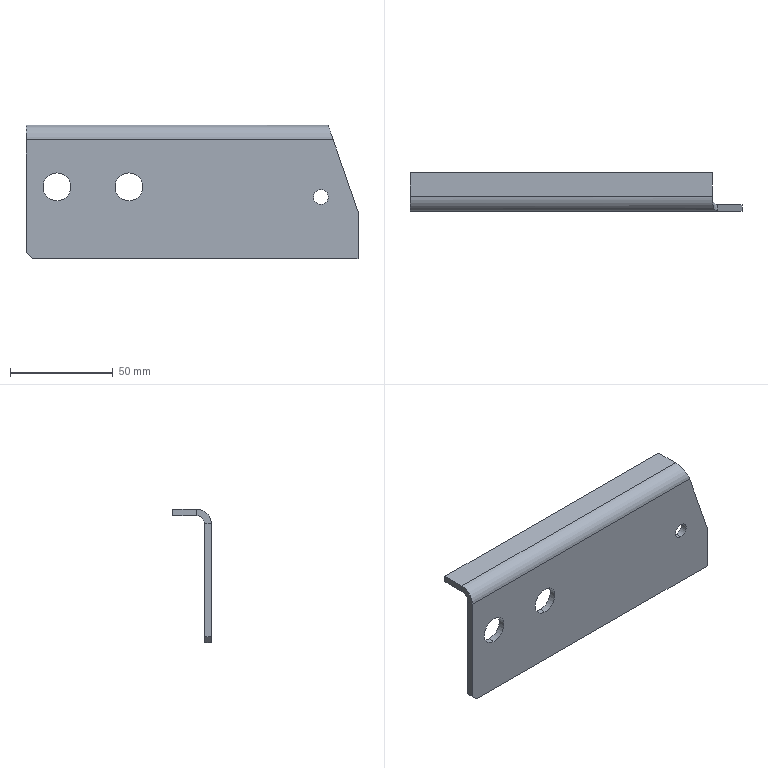Part | SolidWorks | features ICE 3, BreakCorner 1, EdgeFlange 1, FlatPattern 1, SMBaseFlange 1, SheetMetal 1 | 1 solid | 22 faces | box 161.2 x 18.8 x 65 mm | volume 37684 mm3 | plane 13 | cylinder 8 | spline 1 | commonest cylinder face diameters 13.5 x4 7.2 x2 8 x1 14.4 x1
STEP:
#1=CARTESIAN_POINT('',(62.6,-3.2,-6.1));
#2=VERTEX_POINT('',#1);
#3=CARTESIAN_POINT('',(62.6,-3.2,1.1));
#4=VERTEX_POINT('',#3);
#5=CARTESIAN_POINT('',(62.6,-3.2,-2.5));
#6=DIRECTION('',(0.,1.,0.));
#7=DIRECTION('',(0.,0.,1.));
#8=AXIS2_PLACEMENT_3D('',#5,#6,#7);
#9=CIRCLE('',#8,3.6);
#10=EDGE_CURVE('',#2,#4,#9,.T.);
#11=ORIENTED_EDGE('',*,*,#10,.F.);
#12=CARTESIAN_POINT('',(62.6,0.,-6.1));
#13=VERTEX_POINT('',#12);
#14=CARTESIAN_POINT('',(62.6,-10.,-6.1));
#15=DIRECTION('',(0.,1.,0.));
#16=VECTOR('',#15,1000.);
#17=LINE('',#14,#16);
#18=EDGE_CURVE('',#2,#13,#17,.T.);
#19=ORIENTED_EDGE('',*,*,#18,.T.);
#20=CARTESIAN_POINT('',(62.6,0.,1.1));
#21=VERTEX_POINT('',#20);
#22=CARTESIAN_POINT('',(62.6,0.,-2.5));
#23=DIRECTION('',(0.,1.,0.));
#24=DIRECTION('',(0.,0.,1.));
#25=AXIS2_PLACEMENT_3D('',#22,#23,#24);
#26=CIRCLE('',#25,3.6);
#27=EDGE_CURVE('',#13,#21,#26,.T.);
#28=ORIENTED_EDGE('',*,*,#27,.T.);
#29=CARTESIAN_POINT('',(62.6,-10.,1.1));
#30=DIRECTION('',(0.,1.,0.));
#31=VECTOR('',#30,1000.);
#32=LINE('',#29,#31);
#33=EDGE_CURVE('',#4,#21,#32,.T.);
#34=ORIENTED_EDGE('',*,*,#33,.F.);
#35=EDGE_LOOP('',(#11,#19,#28,#34));
#36=FACE_OUTER_BOUND('',#35,.T.);
#37=CARTESIAN_POINT('',(62.6,-10.,-2.5));
#38=DIRECTION('',(0.,1.,0.));
#39=DIRECTION('',(0.,0.,1.));
#40=AXIS2_PLACEMENT_3D('',#37,#38,#39);
#41=CYLINDRICAL_SURFACE('',#40,3.6);
#42=ADVANCED_FACE('',(#36),#41,.F.);
#43=CARTESIAN_POINT('',(-30.6,-3.2,-4.25));
#44=VERTEX_POINT('',#43);
#45=CARTESIAN_POINT('',(-30.6,-3.2,9.25));
#46=VERTEX_POINT('',#45);
#47=CARTESIAN_POINT('',(-30.6,-3.2,2.5));
#48=DIRECTION('',(0.,1.,0.));
#49=DIRECTION('',(0.,0.,1.));
#50=AXIS2_PLACEMENT_3D('',#47,#48,#49);
#51=CIRCLE('',#50,6.75);
#52=EDGE_CURVE('',#44,#46,#51,.T.);
#53=ORIENTED_EDGE('',*,*,#52,.F.);
#54=CARTESIAN_POINT('',(-30.6,0.,-4.25));
#55=VERTEX_POINT('',#54);
#56=CARTESIAN_POINT('',(-30.6,-10.,-4.25));
#57=DIRECTION('',(0.,1.,0.));
#58=VECTOR('',#57,1000.);
#59=LINE('',#56,#58);
#60=EDGE_CURVE('',#44,#55,#59,.T.);
#61=ORIENTED_EDGE('',*,*,#60,.T.);
#62=CARTESIAN_POINT('',(-30.6,0.,9.25));
#63=VERTEX_POINT('',#62);
#64=CARTESIAN_POINT('',(-30.6,0.,2.5));
#65=DIRECTION('',(0.,1.,0.));
#66=DIRECTION('',(0.,0.,1.));
#67=AXIS2_PLACEMENT_3D('',#64,#65,#66);
#68=CIRCLE('',#67,6.75);
#69=EDGE_CURVE('',#55,#63,#68,.T.);
#70=ORIENTED_EDGE('',*,*,#69,.T.);
#71=CARTESIAN_POINT('',(-30.6,-10.,9.25));
#72=DIRECTION('',(0.,1.,0.));
#73=VECTOR('',#72,1000.);
#74=LINE('',#71,#73);
#75=EDGE_CURVE('',#46,#63,#74,.T.);
#76=ORIENTED_EDGE('',*,*,#75,.F.);
#77=EDGE_LOOP('',(#53,#61,#70,#76));
#78=FACE_OUTER_BOUND('',#77,.T.);
#79=CARTESIAN_POINT('',(-30.6,-10.,2.5));
#80=DIRECTION('',(0.,1.,0.));
#81=DIRECTION('',(0.,0.,1.));
#82=AXIS2_PLACEMENT_3D('',#79,#80,#81);
#83=CYLINDRICAL_SURFACE('',#82,6.75);
#84=ADVANCED_FACE('',(#78),#83,.F.);
#85=CARTESIAN_POINT('',(-65.6,-3.2,-4.25));
#86=VERTEX_POINT('',#85);
#87=CARTESIAN_POINT('',(-65.6,-3.2,9.25));
#88=VERTEX_POINT('',#87);
#89=CARTESIAN_POINT('',(-65.6,-3.2,2.5));
#90=DIRECTION('',(0.,1.,0.));
#91=DIRECTION('',(0.,0.,1.));
#92=AXIS2_PLACEMENT_3D('',#89,#90,#91);
#93=CIRCLE('',#92,6.75);
#94=EDGE_CURVE('',#86,#88,#93,.T.);
#95=ORIENTED_EDGE('',*,*,#94,.F.);
#96=CARTESIAN_POINT('',(-65.6,0.,-4.25));
#97=VERTEX_POINT('',#96);
#98=CARTESIAN_POINT('',(-65.6,-10.,-4.25));
#99=DIRECTION('',(0.,1.,0.));
#100=VECTOR('',#99,1000.);
#101=LINE('',#98,#100);
#102=EDGE_CURVE('',#86,#97,#101,.T.);
#103=ORIENTED_EDGE('',*,*,#102,.T.);
#104=CARTESIAN_POINT('',(-65.6,0.,9.25));
#105=VERTEX_POINT('',#104);
#106=CARTESIAN_POINT('',(-65.6,0.,2.5));
#107=DIRECTION('',(0.,1.,0.));
#108=DIRECTION('',(0.,0.,1.));
#109=AXIS2_PLACEMENT_3D('',#106,#107,#108);
#110=CIRCLE('',#109,6.75);
#111=EDGE_CURVE('',#97,#105,#110,.T.);
#112=ORIENTED_EDGE('',*,*,#111,.T.);
#113=CARTESIAN_POINT('',(-65.6,-10.,9.25));
#114=DIRECTION('',(0.,1.,0.));
#115=VECTOR('',#114,1000.);
#116=LINE('',#113,#115);
#117=EDGE_CURVE('',#88,#105,#116,.T.);
#118=ORIENTED_EDGE('',*,*,#117,.F.);
#119=EDGE_LOOP('',(#95,#103,#112,#118));
#120=FACE_OUTER_BOUND('',#119,.T.);
#121=CARTESIAN_POINT('',(-65.6,-10.,2.5));
#122=DIRECTION('',(0.,1.,0.));
#123=DIRECTION('',(0.,0.,1.));
#124=AXIS2_PLACEMENT_3D('',#121,#122,#123);
#125=CYLINDRICAL_SURFACE('',#124,6.75);
#126=ADVANCED_FACE('',(#120),#125,.F.);
#127=CARTESIAN_POINT('',(80.6,0.,-9.6));
#128=VERTEX_POINT('',#127);
#129=CARTESIAN_POINT('',(80.6,0.,-32.5));
#130=VERTEX_POINT('',#129);
#131=CARTESIAN_POINT('',(80.6,0.,-32.5));
#132=DIRECTION('',(0.,0.,-1.));
#133=VECTOR('',#132,1000.);
#134=LINE('',#131,#133);
#135=EDGE_CURVE('',#128,#130,#134,.T.);
#136=ORIENTED_EDGE('',*,*,#135,.F.);
#137=CARTESIAN_POINT('',(80.6,-3.2,-9.6));
#138=VERTEX_POINT('',#137);
#139=CARTESIAN_POINT('',(80.6,0.,-9.6));
#140=DIRECTION('',(0.,-1.,0.));
#141=VECTOR('',#140,1000.);
#142=LINE('',#139,#141);
#143=EDGE_CURVE('',#128,#138,#142,.T.);
#144=ORIENTED_EDGE('',*,*,#143,.T.);
#145=CARTESIAN_POINT('',(80.6,-3.2,-32.5));
#146=VERTEX_POINT('',#145);
#147=CARTESIAN_POINT('',(80.6,-3.2,-32.5));
#148=DIRECTION('',(0.,0.,-1.));
#149=VECTOR('',#148,1000.);
#150=LINE('',#147,#149);
#151=EDGE_CURVE('',#138,#146,#150,.T.);
#152=ORIENTED_EDGE('',*,*,#151,.T.);
#153=CARTESIAN_POINT('',(80.6,-3.2,-32.5));
#154=DIRECTION('',(0.,1.,0.));
#155=VECTOR('',#154,1000.);
#156=LINE('',#153,#155);
#157=EDGE_CURVE('',#146,#130,#156,.T.);
#158=ORIENTED_EDGE('',*,*,#157,.T.);
#159=EDGE_LOOP('',(#136,#144,#152,#158));
#160=FACE_OUTER_BOUND('',#159,.T.);
#161=CARTESIAN_POINT('',(80.6,-3.2,-32.5));
#162=DIRECTION('',(1.,0.,0.));
#163=DIRECTION('',(0.,0.,-1.));
#164=AXIS2_PLACEMENT_3D('',#161,#162,#163);
#165=PLANE('',#164);
#166=ADVANCED_FACE('',(#160),#165,.T.);
#167=CARTESIAN_POINT('',(62.6,-3.2,-2.5));
#168=DIRECTION('',(0.,1.,0.));
#169=DIRECTION('',(0.,0.,1.));
#170=AXIS2_PLACEMENT_3D('',#167,#168,#169);
#171=CIRCLE('',#170,3.6);
#172=EDGE_CURVE('',#4,#2,#171,.T.);
#173=ORIENTED_EDGE('',*,*,#172,.T.);
#174=ORIENTED_EDGE('',*,*,#10,.T.);
#175=EDGE_LOOP('',(#173,#174));
#176=FACE_BOUND('',#175,.T.);
#177=CARTESIAN_POINT('',(-65.6,-3.2,2.5));
#178=DIRECTION('',(0.,1.,0.));
#179=DIRECTION('',(0.,0.,1.));
#180=AXIS2_PLACEMENT_3D('',#177,#178,#179);
#181=CIRCLE('',#180,6.75);
#182=EDGE_CURVE('',#88,#86,#181,.T.);
#183=ORIENTED_EDGE('',*,*,#182,.T.);
#184=ORIENTED_EDGE('',*,*,#94,.T.);
#185=EDGE_LOOP('',(#183,#184));
#186=FACE_BOUND('',#185,.T.);
#187=CARTESIAN_POINT('',(-30.6,-3.2,2.5));
#188=DIRECTION('',(0.,1.,0.));
#189=DIRECTION('',(0.,0.,1.));
#190=AXIS2_PLACEMENT_3D('',#187,#188,#189);
#191=CIRCLE('',#190,6.75);
#192=EDGE_CURVE('',#46,#44,#191,.T.);
#193=ORIENTED_EDGE('',*,*,#192,.T.);
#194=ORIENTED_EDGE('',*,*,#52,.T.);
#195=EDGE_LOOP('',(#193,#194));
#196=FACE_BOUND('',#195,.T.);
#197=CARTESIAN_POINT('',(-80.6,-3.2,-29.5));
#198=VERTEX_POINT('',#197);
#199=CARTESIAN_POINT('',(-80.6,-3.2,25.3));
#200=VERTEX_POINT('',#199);
#201=CARTESIAN_POINT('',(-80.6,-3.2,-32.5));
#202=DIRECTION('',(0.,0.,1.));
#203=VECTOR('',#202,1000.);
#204=LINE('',#201,#203);
#205=EDGE_CURVE('',#198,#200,#204,.T.);
#206=ORIENTED_EDGE('',*,*,#205,.F.);
#207=CARTESIAN_POINT('',(-77.6,-3.2,-32.5));
#208=VERTEX_POINT('',#207);
#209=CARTESIAN_POINT('',(-77.6,-3.2,-32.5));
#210=DIRECTION('',(0.7071,0.,-0.7071));
#211=VECTOR('',#210,1000.);
#212=LINE('',#209,#211);
#213=EDGE_CURVE('',#198,#208,#212,.T.);
#214=ORIENTED_EDGE('',*,*,#213,.T.);
#215=CARTESIAN_POINT('',(-80.6,-3.2,-32.5));
#216=DIRECTION('',(-1.,0.,0.));
#217=VECTOR('',#216,1000.);
#218=LINE('',#215,#217);
#219=EDGE_CURVE('',#146,#208,#218,.T.);
#220=ORIENTED_EDGE('',*,*,#219,.F.);
#221=ORIENTED_EDGE('',*,*,#151,.F.);
#222=CARTESIAN_POINT('',(68.58,-3.2,25.3));
#223=VERTEX_POINT('',#222);
#224=CARTESIAN_POINT('',(69.097,-3.2,23.798));
#225=DIRECTION('',(0.3256,0.,-0.9455));
#226=VECTOR('',#225,1000.);
#227=LINE('',#224,#226);
#228=EDGE_CURVE('',#223,#138,#227,.T.);
#229=ORIENTED_EDGE('',*,*,#228,.F.);
#230=CARTESIAN_POINT('',(80.6,-3.2,25.3));
#231=DIRECTION('',(-1.,0.,0.));
#232=VECTOR('',#231,1000.);
#233=LINE('',#230,#232);
#234=EDGE_CURVE('',#223,#200,#233,.T.);
#235=ORIENTED_EDGE('',*,*,#234,.T.);
#236=EDGE_LOOP('',(#206,#214,#220,#221,#229,#235));
#237=FACE_OUTER_BOUND('',#236,.T.);
#238=CARTESIAN_POINT('',(0.,-3.2,0.));
#239=DIRECTION('',(0.,1.,0.));
#240=DIRECTION('',(0.,0.,1.));
#241=AXIS2_PLACEMENT_3D('',#238,#239,#240);
#242=PLANE('',#241);
#243=ADVANCED_FACE('',(#176,#186,#196,#237),#242,.F.);
#244=CARTESIAN_POINT('',(62.6,0.,-2.5));
#245=DIRECTION('',(0.,1.,0.));
#246=DIRECTION('',(0.,0.,1.));
#247=AXIS2_PLACEMENT_3D('',#244,#245,#246);
#248=CIRCLE('',#247,3.6);
#249=EDGE_CURVE('',#21,#13,#248,.T.);
#250=ORIENTED_EDGE('',*,*,#249,.F.);
#251=ORIENTED_EDGE('',*,*,#27,.F.);
#252=EDGE_LOOP('',(#250,#251));
#253=FACE_BOUND('',#252,.T.);
#254=CARTESIAN_POINT('',(-30.6,0.,2.5));
#255=DIRECTION('',(0.,1.,0.));
#256=DIRECTION('',(0.,0.,1.));
#257=AXIS2_PLACEMENT_3D('',#254,#255,#256);
#258=CIRCLE('',#257,6.75);
#259=EDGE_CURVE('',#63,#55,#258,.T.);
#260=ORIENTED_EDGE('',*,*,#259,.F.);
#261=ORIENTED_EDGE('',*,*,#69,.F.);
#262=EDGE_LOOP('',(#260,#261));
#263=FACE_BOUND('',#262,.T.);
#264=CARTESIAN_POINT('',(-65.6,0.,2.5));
#265=DIRECTION('',(0.,1.,0.));
#266=DIRECTION('',(0.,0.,1.));
#267=AXIS2_PLACEMENT_3D('',#264,#265,#266);
#268=CIRCLE('',#267,6.75);
#269=EDGE_CURVE('',#105,#97,#268,.T.);
#270=ORIENTED_EDGE('',*,*,#269,.F.);
#271=ORIENTED_EDGE('',*,*,#111,.F.);
#272=EDGE_LOOP('',(#270,#271));
#273=FACE_BOUND('',#272,.T.);
#274=CARTESIAN_POINT('',(-77.6,0.,-32.5));
#275=VERTEX_POINT('',#274);
#276=CARTESIAN_POINT('',(-80.6,0.,-32.5));
#277=DIRECTION('',(-1.,0.,0.));
#278=VECTOR('',#277,1000.);
#279=LINE('',#276,#278);
#280=EDGE_CURVE('',#130,#275,#279,.T.);
#281=ORIENTED_EDGE('',*,*,#280,.T.);
#282=CARTESIAN_POINT('',(-80.6,0.,-29.5));
#283=VERTEX_POINT('',#282);
#284=CARTESIAN_POINT('',(-55.05,0.,-55.05));
#285=DIRECTION('',(-0.7071,0.,0.7071));
#286=VECTOR('',#285,1000.);
#287=LINE('',#284,#286);
#288=EDGE_CURVE('',#275,#283,#287,.T.);
#289=ORIENTED_EDGE('',*,*,#288,.T.);
#290=CARTESIAN_POINT('',(-80.6,0.,25.3));
#291=VERTEX_POINT('',#290);
#292=CARTESIAN_POINT('',(-80.6,0.,-32.5));
#293=DIRECTION('',(0.,0.,1.));
#294=VECTOR('',#293,1000.);
#295=LINE('',#292,#294);
#296=EDGE_CURVE('',#283,#291,#295,.T.);
#297=ORIENTED_EDGE('',*,*,#296,.T.);
#298=CARTESIAN_POINT('',(68.58,0.,25.3));
#299=VERTEX_POINT('',#298);
#300=CARTESIAN_POINT('',(80.6,0.,25.3));
#301=DIRECTION('',(-1.,0.,0.));
#302=VECTOR('',#301,1000.);
#303=LINE('',#300,#302);
#304=EDGE_CURVE('',#299,#291,#303,.T.);
#305=ORIENTED_EDGE('',*,*,#304,.F.);
#306=CARTESIAN_POINT('',(69.097,0.,23.798));
#307=DIRECTION('',(0.3256,0.,-0.9455));
#308=VECTOR('',#307,1000.);
#309=LINE('',#306,#308);
#310=EDGE_CURVE('',#299,#128,#309,.T.);
#311=ORIENTED_EDGE('',*,*,#310,.T.);
#312=ORIENTED_EDGE('',*,*,#135,.T.);
#313=EDGE_LOOP('',(#281,#289,#297,#305,#311,#312));
#314=FACE_OUTER_BOUND('',#313,.T.);
#315=CARTESIAN_POINT('',(0.,0.,0.));
#316=DIRECTION('',(0.,1.,0.));
#317=DIRECTION('',(0.,0.,1.));
#318=AXIS2_PLACEMENT_3D('',#315,#316,#317);
#319=PLANE('',#318);
#320=ADVANCED_FACE('',(#253,#263,#273,#314),#319,.T.);
#321=ORIENTED_EDGE('',*,*,#234,.F.);
#322=CARTESIAN_POINT('',(66.1,4.,32.5));
#323=VERTEX_POINT('',#322);
#324=CARTESIAN_POINT('',(68.58,-3.2,25.3));
#325=CARTESIAN_POINT('',(67.127,-3.2,29.518));
#326=CARTESIAN_POINT('',(66.1,-0.2177,32.5));
#327=CARTESIAN_POINT('',(66.1,4.,32.5));
#328=(BOUNDED_CURVE()B_SPLINE_CURVE(3,(#324,#325,#326,#327),.UNSPECIFIED.,.F.,.F.)B_SPLINE_CURVE_WITH_KNOTS((4,4),(1.571,3.142),.UNSPECIFIED.)CURVE()GEOMETRIC_REPRESENTATION_ITEM()RATIONAL_B_SPLINE_CURVE((1.,0.8047,0.8047,1.))REPRESENTATION_ITEM(''));
#329=EDGE_CURVE('',#223,#323,#328,.T.);
#330=ORIENTED_EDGE('',*,*,#329,.T.);
#331=CARTESIAN_POINT('',(-80.6,4.,32.5));
#332=VERTEX_POINT('',#331);
#333=CARTESIAN_POINT('',(0.,4.,32.5));
#334=DIRECTION('',(1.,0.,0.));
#335=VECTOR('',#334,1000.);
#336=LINE('',#333,#335);
#337=EDGE_CURVE('',#332,#323,#336,.T.);
#338=ORIENTED_EDGE('',*,*,#337,.F.);
#339=CARTESIAN_POINT('',(-80.6,4.,25.3));
#340=DIRECTION('',(-1.,0.,0.));
#341=DIRECTION('',(0.,0.,-1.));
#342=AXIS2_PLACEMENT_3D('',#339,#340,#341);
#343=CIRCLE('',#342,7.2);
#344=EDGE_CURVE('',#200,#332,#343,.T.);
#345=ORIENTED_EDGE('',*,*,#344,.F.);
#346=EDGE_LOOP('',(#321,#330,#338,#345));
#347=FACE_OUTER_BOUND('',#346,.T.);
#348=CARTESIAN_POINT('',(80.6,4.,25.3));
#349=DIRECTION('',(1.,0.,0.));
#350=DIRECTION('',(0.,0.,1.));
#351=AXIS2_PLACEMENT_3D('',#348,#349,#350);
#352=CYLINDRICAL_SURFACE('',#351,7.2);
#353=ADVANCED_FACE('',(#347),#352,.T.);
#354=CARTESIAN_POINT('',(66.1,4.,29.3));
#355=VERTEX_POINT('',#354);
#356=CARTESIAN_POINT('',(68.58,0.,25.3));
#357=CARTESIAN_POINT('',(67.127,0.,27.643));
#358=CARTESIAN_POINT('',(66.1,1.657,29.3));
#359=CARTESIAN_POINT('',(66.1,4.,29.3));
#360=(BOUNDED_CURVE()B_SPLINE_CURVE(3,(#356,#357,#358,#359),.UNSPECIFIED.,.F.,.F.)B_SPLINE_CURVE_WITH_KNOTS((4,4),(1.571,3.142),.UNSPECIFIED.)CURVE()GEOMETRIC_REPRESENTATION_ITEM()RATIONAL_B_SPLINE_CURVE((1.,0.8047,0.8047,1.))REPRESENTATION_ITEM(''));
#361=EDGE_CURVE('',#299,#355,#360,.T.);
#362=ORIENTED_EDGE('',*,*,#361,.F.);
#363=ORIENTED_EDGE('',*,*,#304,.T.);
#364=CARTESIAN_POINT('',(-80.6,4.,29.3));
#365=VERTEX_POINT('',#364);
#366=CARTESIAN_POINT('',(-80.6,4.,25.3));
#367=DIRECTION('',(-1.,0.,0.));
#368=DIRECTION('',(0.,0.,-1.));
#369=AXIS2_PLACEMENT_3D('',#366,#367,#368);
#370=CIRCLE('',#369,4.);
#371=EDGE_CURVE('',#291,#365,#370,.T.);
#372=ORIENTED_EDGE('',*,*,#371,.T.);
#373=CARTESIAN_POINT('',(-80.6,4.,29.3));
#374=DIRECTION('',(1.,0.,0.));
#375=VECTOR('',#374,1000.);
#376=LINE('',#373,#375);
#377=EDGE_CURVE('',#365,#355,#376,.T.);
#378=ORIENTED_EDGE('',*,*,#377,.T.);
#379=EDGE_LOOP('',(#362,#363,#372,#378));
#380=FACE_OUTER_BOUND('',#379,.T.);
#381=CARTESIAN_POINT('',(80.6,4.,25.3));
#382=DIRECTION('',(1.,0.,0.));
#383=DIRECTION('',(0.,0.,1.));
#384=AXIS2_PLACEMENT_3D('',#381,#382,#383);
#385=CYLINDRICAL_SURFACE('',#384,4.);
#386=ADVANCED_FACE('',(#380),#385,.F.);
#387=ORIENTED_EDGE('',*,*,#337,.T.);
#388=CARTESIAN_POINT('',(66.1,15.6,32.5));
#389=VERTEX_POINT('',#388);
#390=CARTESIAN_POINT('',(66.1,218.532,32.5));
#391=DIRECTION('',(0.,-1.,0.));
#392=VECTOR('',#391,1000.);
#393=LINE('',#390,#392);
#394=EDGE_CURVE('',#389,#323,#393,.T.);
#395=ORIENTED_EDGE('',*,*,#394,.F.);
#396=CARTESIAN_POINT('',(-80.6,15.6,32.5));
#397=VERTEX_POINT('',#396);
#398=CARTESIAN_POINT('',(0.,15.6,32.5));
#399=DIRECTION('',(-1.,0.,0.));
#400=VECTOR('',#399,1000.);
#401=LINE('',#398,#400);
#402=EDGE_CURVE('',#389,#397,#401,.T.);
#403=ORIENTED_EDGE('',*,*,#402,.T.);
#404=CARTESIAN_POINT('',(-80.6,0.,32.5));
#405=DIRECTION('',(0.,-1.,0.));
#406=VECTOR('',#405,1000.);
#407=LINE('',#404,#406);
#408=EDGE_CURVE('',#397,#332,#407,.T.);
#409=ORIENTED_EDGE('',*,*,#408,.T.);
#410=EDGE_LOOP('',(#387,#395,#403,#409));
#411=FACE_OUTER_BOUND('',#410,.T.);
#412=CARTESIAN_POINT('',(0.,0.,32.5));
#413=DIRECTION('',(0.,0.,1.));
#414=DIRECTION('',(1.,0.,0.));
#415=AXIS2_PLACEMENT_3D('',#412,#413,#414);
#416=PLANE('',#415);
#417=ADVANCED_FACE('',(#411),#416,.T.);
#418=CARTESIAN_POINT('',(66.1,15.6,29.3));
#419=VERTEX_POINT('',#418);
#420=CARTESIAN_POINT('',(66.1,0.,29.3));
#421=DIRECTION('',(0.,-1.,0.));
#422=VECTOR('',#421,1000.);
#423=LINE('',#420,#422);
#424=EDGE_CURVE('',#419,#355,#423,.T.);
#425=ORIENTED_EDGE('',*,*,#424,.T.);
#426=ORIENTED_EDGE('',*,*,#377,.F.);
#427=CARTESIAN_POINT('',(-80.6,15.6,29.3));
#428=VERTEX_POINT('',#427);
#429=CARTESIAN_POINT('',(-80.6,15.6,29.3));
#430=DIRECTION('',(0.,-1.,0.));
#431=VECTOR('',#430,1000.);
#432=LINE('',#429,#431);
#433=EDGE_CURVE('',#428,#365,#432,.T.);
#434=ORIENTED_EDGE('',*,*,#433,.F.);
#435=CARTESIAN_POINT('',(80.6,15.6,29.3));
#436=DIRECTION('',(-1.,0.,0.));
#437=VECTOR('',#436,1000.);
#438=LINE('',#435,#437);
#439=EDGE_CURVE('',#419,#428,#438,.T.);
#440=ORIENTED_EDGE('',*,*,#439,.F.);
#441=EDGE_LOOP('',(#425,#426,#434,#440));
#442=FACE_OUTER_BOUND('',#441,.T.);
#443=CARTESIAN_POINT('',(0.,0.,29.3));
#444=DIRECTION('',(0.,0.,1.));
#445=DIRECTION('',(1.,0.,0.));
#446=AXIS2_PLACEMENT_3D('',#443,#444,#445);
#447=PLANE('',#446);
#448=ADVANCED_FACE('',(#442),#447,.F.);
#449=CARTESIAN_POINT('',(66.1,15.6,32.5));
#450=DIRECTION('',(0.,0.,-1.));
#451=VECTOR('',#450,1000.);
#452=LINE('',#449,#451);
#453=EDGE_CURVE('',#389,#419,#452,.T.);
#454=ORIENTED_EDGE('',*,*,#453,.T.);
#455=ORIENTED_EDGE('',*,*,#439,.T.);
#456=CARTESIAN_POINT('',(-80.6,15.6,32.5));
#457=DIRECTION('',(0.,0.,-1.));
#458=VECTOR('',#457,1000.);
#459=LINE('',#456,#458);
#460=EDGE_CURVE('',#397,#428,#459,.T.);
#461=ORIENTED_EDGE('',*,*,#460,.F.);
#462=ORIENTED_EDGE('',*,*,#402,.F.);
#463=EDGE_LOOP('',(#454,#455,#461,#462));
#464=FACE_OUTER_BOUND('',#463,.T.);
#465=CARTESIAN_POINT('',(80.6,15.6,32.5));
#466=DIRECTION('',(0.,-1.,0.));
#467=DIRECTION('',(0.,0.,-1.));
#468=AXIS2_PLACEMENT_3D('',#465,#466,#467);
#469=PLANE('',#468);
#470=ADVANCED_FACE('',(#464),#469,.F.);
#471=ORIENTED_EDGE('',*,*,#296,.F.);
#472=CARTESIAN_POINT('',(-80.6,-3.2,-29.5));
#473=DIRECTION('',(0.,-1.,0.));
#474=VECTOR('',#473,1000.);
#475=LINE('',#472,#474);
#476=EDGE_CURVE('',#283,#198,#475,.T.);
#477=ORIENTED_EDGE('',*,*,#476,.T.);
#478=ORIENTED_EDGE('',*,*,#205,.T.);
#479=CARTESIAN_POINT('',(-80.6,0.,25.3));
#480=DIRECTION('',(0.,-1.,0.));
#481=VECTOR('',#480,1000.);
#482=LINE('',#479,#481);
#483=EDGE_CURVE('',#291,#200,#482,.T.);
#484=ORIENTED_EDGE('',*,*,#483,.F.);
#485=EDGE_LOOP('',(#471,#477,#478,#484));
#486=FACE_OUTER_BOUND('',#485,.T.);
#487=CARTESIAN_POINT('',(-80.6,-3.2,-32.5));
#488=DIRECTION('',(-1.,0.,0.));
#489=DIRECTION('',(0.,0.,1.));
#490=AXIS2_PLACEMENT_3D('',#487,#488,#489);
#491=PLANE('',#490);
#492=ADVANCED_FACE('',(#486),#491,.T.);
#493=ORIENTED_EDGE('',*,*,#219,.T.);
#494=CARTESIAN_POINT('',(-77.6,-3.2,-32.5));
#495=DIRECTION('',(0.,1.,0.));
#496=VECTOR('',#495,1000.);
#497=LINE('',#494,#496);
#498=EDGE_CURVE('',#208,#275,#497,.T.);
#499=ORIENTED_EDGE('',*,*,#498,.T.);
#500=ORIENTED_EDGE('',*,*,#280,.F.);
#501=ORIENTED_EDGE('',*,*,#157,.F.);
#502=EDGE_LOOP('',(#493,#499,#500,#501));
#503=FACE_OUTER_BOUND('',#502,.T.);
#504=CARTESIAN_POINT('',(-80.6,-3.2,-32.5));
#505=DIRECTION('',(0.,0.,-1.));
#506=DIRECTION('',(-1.,0.,0.));
#507=AXIS2_PLACEMENT_3D('',#504,#505,#506);
#508=PLANE('',#507);
#509=ADVANCED_FACE('',(#503),#508,.T.);
#510=CARTESIAN_POINT('',(-80.6,4.,32.5));
#511=DIRECTION('',(0.,0.,1.));
#512=VECTOR('',#511,1000.);
#513=LINE('',#510,#512);
#514=EDGE_CURVE('',#365,#332,#513,.T.);
#515=ORIENTED_EDGE('',*,*,#514,.F.);
#516=ORIENTED_EDGE('',*,*,#371,.F.);
#517=ORIENTED_EDGE('',*,*,#483,.T.);
#518=ORIENTED_EDGE('',*,*,#344,.T.);
#519=EDGE_LOOP('',(#515,#516,#517,#518));
#520=FACE_OUTER_BOUND('',#519,.T.);
#521=CARTESIAN_POINT('',(-80.6,4.,25.3));
#522=DIRECTION('',(-1.,0.,0.));
#523=DIRECTION('',(0.,0.,1.));
#524=AXIS2_PLACEMENT_3D('',#521,#522,#523);
#525=PLANE('',#524);
#526=ADVANCED_FACE('',(#520),#525,.T.);
#527=ORIENTED_EDGE('',*,*,#514,.T.);
#528=ORIENTED_EDGE('',*,*,#408,.F.);
#529=ORIENTED_EDGE('',*,*,#460,.T.);
#530=ORIENTED_EDGE('',*,*,#433,.T.);
#531=EDGE_LOOP('',(#527,#528,#529,#530));
#532=FACE_OUTER_BOUND('',#531,.T.);
#533=CARTESIAN_POINT('',(-80.6,15.6,32.5));
#534=DIRECTION('',(1.,0.,0.));
#535=DIRECTION('',(0.,0.,-1.));
#536=AXIS2_PLACEMENT_3D('',#533,#534,#535);
#537=PLANE('',#536);
#538=ADVANCED_FACE('',(#532),#537,.F.);
#539=ORIENTED_EDGE('',*,*,#102,.F.);
#540=ORIENTED_EDGE('',*,*,#182,.F.);
#541=ORIENTED_EDGE('',*,*,#117,.T.);
#542=ORIENTED_EDGE('',*,*,#269,.T.);
#543=EDGE_LOOP('',(#539,#540,#541,#542));
#544=FACE_OUTER_BOUND('',#543,.T.);
#545=CARTESIAN_POINT('',(-65.6,-10.,2.5));
#546=DIRECTION('',(0.,1.,0.));
#547=DIRECTION('',(0.,0.,1.));
#548=AXIS2_PLACEMENT_3D('',#545,#546,#547);
#549=CYLINDRICAL_SURFACE('',#548,6.75);
#550=ADVANCED_FACE('',(#544),#549,.F.);
#551=ORIENTED_EDGE('',*,*,#60,.F.);
#552=ORIENTED_EDGE('',*,*,#192,.F.);
#553=ORIENTED_EDGE('',*,*,#75,.T.);
#554=ORIENTED_EDGE('',*,*,#259,.T.);
#555=EDGE_LOOP('',(#551,#552,#553,#554));
#556=FACE_OUTER_BOUND('',#555,.T.);
#557=CARTESIAN_POINT('',(-30.6,-10.,2.5));
#558=DIRECTION('',(0.,1.,0.));
#559=DIRECTION('',(0.,0.,1.));
#560=AXIS2_PLACEMENT_3D('',#557,#558,#559);
#561=CYLINDRICAL_SURFACE('',#560,6.75);
#562=ADVANCED_FACE('',(#556),#561,.F.);
#563=ORIENTED_EDGE('',*,*,#453,.F.);
#564=ORIENTED_EDGE('',*,*,#394,.T.);
#565=CARTESIAN_POINT('',(66.1,4.,32.5));
#566=DIRECTION('',(0.,0.,-1.));
#567=VECTOR('',#566,1000.);
#568=LINE('',#565,#567);
#569=EDGE_CURVE('',#323,#355,#568,.T.);
#570=ORIENTED_EDGE('',*,*,#569,.T.);
#571=ORIENTED_EDGE('',*,*,#424,.F.);
#572=EDGE_LOOP('',(#563,#564,#570,#571));
#573=FACE_OUTER_BOUND('',#572,.T.);
#574=CARTESIAN_POINT('',(66.1,218.532,32.5));
#575=DIRECTION('',(-1.,0.,0.));
#576=DIRECTION('',(0.,-1.,0.));
#577=AXIS2_PLACEMENT_3D('',#574,#575,#576);
#578=PLANE('',#577);
#579=ADVANCED_FACE('',(#573),#578,.F.);
#580=ORIENTED_EDGE('',*,*,#143,.F.);
#581=ORIENTED_EDGE('',*,*,#310,.F.);
#582=CARTESIAN_POINT('',(68.58,0.,25.3));
#583=DIRECTION('',(0.,-1.,0.));
#584=VECTOR('',#583,1000.);
#585=LINE('',#582,#584);
#586=EDGE_CURVE('',#299,#223,#585,.T.);
#587=ORIENTED_EDGE('',*,*,#586,.T.);
#588=ORIENTED_EDGE('',*,*,#228,.T.);
#589=EDGE_LOOP('',(#580,#581,#587,#588));
#590=FACE_OUTER_BOUND('',#589,.T.);
#591=CARTESIAN_POINT('',(69.097,0.,23.798));
#592=DIRECTION('',(0.9455,0.,0.3256));
#593=DIRECTION('',(0.3256,0.,-0.9455));
#594=AXIS2_PLACEMENT_3D('',#591,#592,#593);
#595=PLANE('',#594);
#596=ADVANCED_FACE('',(#590),#595,.T.);
#597=ORIENTED_EDGE('',*,*,#569,.F.);
#598=ORIENTED_EDGE('',*,*,#329,.F.);
#599=ORIENTED_EDGE('',*,*,#586,.F.);
#600=ORIENTED_EDGE('',*,*,#361,.T.);
#601=EDGE_LOOP('',(#597,#598,#599,#600));
#602=FACE_OUTER_BOUND('',#601,.T.);
#603=CARTESIAN_POINT('',(71.06,4.,18.1));
#604=CARTESIAN_POINT('',(71.06,4.,19.167));
#605=CARTESIAN_POINT('',(71.06,4.,20.233));
#606=CARTESIAN_POINT('',(71.06,4.,21.3));
#607=CARTESIAN_POINT('',(71.06,-10.4,18.1));
#608=CARTESIAN_POINT('',(71.06,-8.267,19.167));
#609=CARTESIAN_POINT('',(71.06,-6.133,20.233));
#610=CARTESIAN_POINT('',(71.06,-4.,21.3));
#611=CARTESIAN_POINT('',(66.1,-10.4,32.5));
#612=CARTESIAN_POINT('',(66.1,-8.267,31.433));
#613=CARTESIAN_POINT('',(66.1,-6.133,30.367));
#614=CARTESIAN_POINT('',(66.1,-4.,29.3));
#615=CARTESIAN_POINT('',(66.1,4.,32.5));
#616=CARTESIAN_POINT('',(66.1,4.,31.433));
#617=CARTESIAN_POINT('',(66.1,4.,30.367));
#618=CARTESIAN_POINT('',(66.1,4.,29.3));
#619=CARTESIAN_POINT('',(66.1,18.4,32.5));
#620=CARTESIAN_POINT('',(66.1,16.267,31.433));
#621=CARTESIAN_POINT('',(66.1,14.133,30.367));
#622=CARTESIAN_POINT('',(66.1,12.,29.3));
#623=CARTESIAN_POINT('',(71.06,18.4,18.1));
#624=CARTESIAN_POINT('',(71.06,16.267,19.167));
#625=CARTESIAN_POINT('',(71.06,14.133,20.233));
#626=CARTESIAN_POINT('',(71.06,12.,21.3));
#627=CARTESIAN_POINT('',(71.06,4.,18.1));
#628=CARTESIAN_POINT('',(71.06,4.,19.167));
#629=CARTESIAN_POINT('',(71.06,4.,20.233));
#630=CARTESIAN_POINT('',(71.06,4.,21.3));
#631=(BOUNDED_SURFACE()B_SPLINE_SURFACE(3,3,((#603,#604,#605,#606),(#607,#608,#609,#610),(#611,#612,#613,#614),(#615,#616,#617,#618),(#619,#620,#621,#622),(#623,#624,#625,#626),(#627,#628,#629,#630)),.UNSPECIFIED.,.T.,.F.,.F.)B_SPLINE_SURFACE_WITH_KNOTS((4,3,4),(4,4),(0.,0.5,1.),(0.,1.),.UNSPECIFIED.)GEOMETRIC_REPRESENTATION_ITEM()RATIONAL_B_SPLINE_SURFACE(((1.,1.,1.,1.),(0.3333,0.3333,0.3333,0.3333),(0.3333,0.3333,0.3333,0.3333),(1.,1.,1.,1.),(0.3333,0.3333,0.3333,0.3333),(0.3333,0.3333,0.3333,0.3333),(1.,1.,1.,1.)))REPRESENTATION_ITEM('')SURFACE());
#632=ADVANCED_FACE('',(#602),#631,.F.);
#633=ORIENTED_EDGE('',*,*,#213,.F.);
#634=ORIENTED_EDGE('',*,*,#476,.F.);
#635=ORIENTED_EDGE('',*,*,#288,.F.);
#636=ORIENTED_EDGE('',*,*,#498,.F.);
#637=EDGE_LOOP('',(#633,#634,#635,#636));
#638=FACE_OUTER_BOUND('',#637,.T.);
#639=CARTESIAN_POINT('',(-77.6,-3.2,-32.5));
#640=DIRECTION('',(0.7071,0.,0.7071));
#641=DIRECTION('',(0.,1.,0.));
#642=AXIS2_PLACEMENT_3D('',#639,#640,#641);
#643=PLANE('',#642);
#644=ADVANCED_FACE('',(#638),#643,.F.);
#645=ORIENTED_EDGE('',*,*,#18,.F.);
#646=ORIENTED_EDGE('',*,*,#172,.F.);
#647=ORIENTED_EDGE('',*,*,#33,.T.);
#648=ORIENTED_EDGE('',*,*,#249,.T.);
#649=EDGE_LOOP('',(#645,#646,#647,#648));
#650=FACE_OUTER_BOUND('',#649,.T.);
#651=CARTESIAN_POINT('',(62.6,-10.,-2.5));
#652=DIRECTION('',(0.,1.,0.));
#653=DIRECTION('',(0.,0.,1.));
#654=AXIS2_PLACEMENT_3D('',#651,#652,#653);
#655=CYLINDRICAL_SURFACE('',#654,3.6);
#656=ADVANCED_FACE('',(#650),#655,.F.);
#657=CLOSED_SHELL('',(#42,#84,#126,#166,#243,#320,#353,#386,#417,#448,#470,#492,#509,#526,#538,#550,#562,#579,#596,#632,#644,#656));
#658=MANIFOLD_SOLID_BREP('',#657);
#659=CARTESIAN_POINT('',(0.,0.,0.));
#660=DIRECTION('',(0.,0.,1.));
#661=DIRECTION('',(1.,0.,0.));
#662=AXIS2_PLACEMENT_3D('',#659,#660,#661);
#663=(LENGTH_UNIT()NAMED_UNIT(*)SI_UNIT(.MILLI.,.METRE.));
#664=UNCERTAINTY_MEASURE_WITH_UNIT(LENGTH_MEASURE(0.00001),#663,'','');
#665=(NAMED_UNIT(*)PLANE_ANGLE_UNIT()SI_UNIT($,.RADIAN.));
#666=(NAMED_UNIT(*)SI_UNIT($,.STERADIAN.)SOLID_ANGLE_UNIT());
#667=(GEOMETRIC_REPRESENTATION_CONTEXT(3)GLOBAL_UNCERTAINTY_ASSIGNED_CONTEXT((#664))GLOBAL_UNIT_ASSIGNED_CONTEXT((#663,#665,#666))REPRESENTATION_CONTEXT('',''));
#668=ADVANCED_BREP_SHAPE_REPRESENTATION('',(#658,#662),#667);